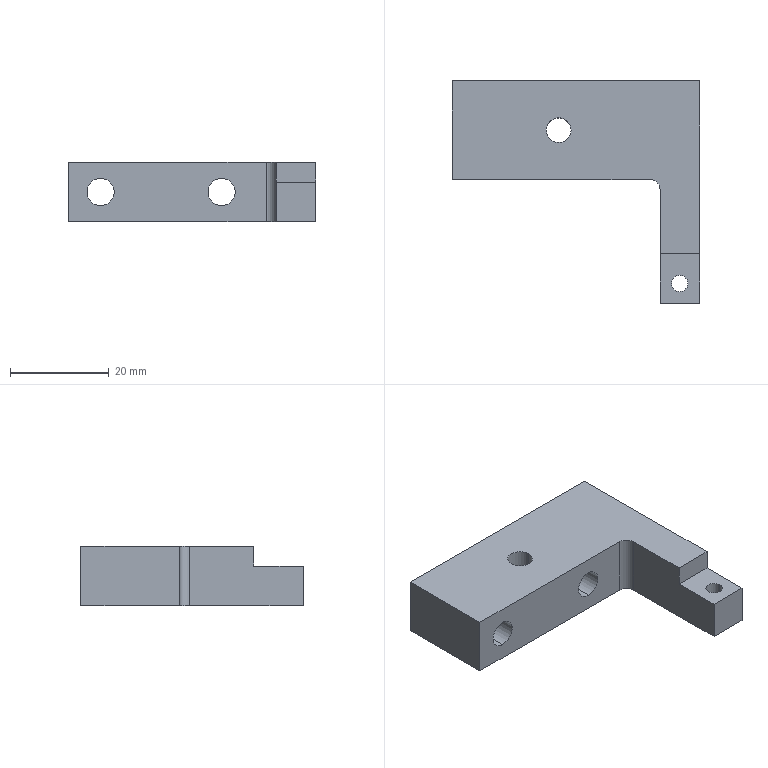Part | STEP file | 11-FG-B05211 | 1 solid | 19 faces | box 50 x 45 x 12 mm | volume 12836 mm3 | plane 10 | cylinder 9 | commonest cylinder face diameters 5.5 x4 3.3 x2 5 x2 4 x1
STEP:
#1=CARTESIAN_POINT('',(24.,10.,0.));
#2=VERTEX_POINT('',#1);
#3=CARTESIAN_POINT('',(19.,10.,0.));
#4=VERTEX_POINT('',#3);
#5=CARTESIAN_POINT('',(21.5,10.,0.));
#6=DIRECTION('',(0.,0.,-1.));
#7=DIRECTION('',(-1.,0.,0.));
#8=AXIS2_PLACEMENT_3D('',#5,#6,#7);
#9=CIRCLE('',#8,2.5);
#10=EDGE_CURVE('',#2,#4,#9,.T.);
#11=ORIENTED_EDGE('',*,*,#10,.T.);
#12=CARTESIAN_POINT('',(19.,10.,12.));
#13=VERTEX_POINT('',#12);
#14=CARTESIAN_POINT('',(19.,10.,12.));
#15=DIRECTION('',(0.,0.,1.));
#16=VECTOR('',#15,1000.);
#17=LINE('',#14,#16);
#18=EDGE_CURVE('',#4,#13,#17,.T.);
#19=ORIENTED_EDGE('',*,*,#18,.T.);
#20=CARTESIAN_POINT('',(24.,10.,12.));
#21=VERTEX_POINT('',#20);
#22=CARTESIAN_POINT('',(21.5,10.,12.));
#23=DIRECTION('',(0.,0.,1.));
#24=DIRECTION('',(1.,0.,0.));
#25=AXIS2_PLACEMENT_3D('',#22,#23,#24);
#26=CIRCLE('',#25,2.5);
#27=EDGE_CURVE('',#13,#21,#26,.T.);
#28=ORIENTED_EDGE('',*,*,#27,.T.);
#29=CARTESIAN_POINT('',(24.,10.,12.));
#30=DIRECTION('',(0.,0.,1.));
#31=VECTOR('',#30,1000.);
#32=LINE('',#29,#31);
#33=EDGE_CURVE('',#2,#21,#32,.T.);
#34=ORIENTED_EDGE('',*,*,#33,.F.);
#35=EDGE_LOOP('',(#11,#19,#28,#34));
#36=FACE_OUTER_BOUND('',#35,.T.);
#37=CARTESIAN_POINT('',(21.5,10.,12.));
#38=DIRECTION('',(0.,0.,1.));
#39=DIRECTION('',(1.,0.,0.));
#40=AXIS2_PLACEMENT_3D('',#37,#38,#39);
#41=CYLINDRICAL_SURFACE('',#40,2.5);
#42=ADVANCED_FACE('',(#36),#41,.F.);
#43=CARTESIAN_POINT('',(31.,20.,8.75));
#44=VERTEX_POINT('',#43);
#45=CARTESIAN_POINT('',(31.,20.,3.25));
#46=VERTEX_POINT('',#45);
#47=CARTESIAN_POINT('',(31.,20.,6.));
#48=DIRECTION('',(0.,-1.,0.));
#49=DIRECTION('',(0.,0.,-1.));
#50=AXIS2_PLACEMENT_3D('',#47,#48,#49);
#51=CIRCLE('',#50,2.75);
#52=EDGE_CURVE('',#44,#46,#51,.T.);
#53=ORIENTED_EDGE('',*,*,#52,.F.);
#54=CARTESIAN_POINT('',(31.,0.,8.75));
#55=VERTEX_POINT('',#54);
#56=CARTESIAN_POINT('',(31.,28.,8.75));
#57=DIRECTION('',(0.,-1.,0.));
#58=VECTOR('',#57,1000.);
#59=LINE('',#56,#58);
#60=EDGE_CURVE('',#44,#55,#59,.T.);
#61=ORIENTED_EDGE('',*,*,#60,.T.);
#62=CARTESIAN_POINT('',(31.,0.,3.25));
#63=VERTEX_POINT('',#62);
#64=CARTESIAN_POINT('',(31.,0.,6.));
#65=DIRECTION('',(0.,-1.,0.));
#66=DIRECTION('',(0.,0.,-1.));
#67=AXIS2_PLACEMENT_3D('',#64,#65,#66);
#68=CIRCLE('',#67,2.75);
#69=EDGE_CURVE('',#55,#63,#68,.T.);
#70=ORIENTED_EDGE('',*,*,#69,.T.);
#71=CARTESIAN_POINT('',(31.,28.,3.25));
#72=DIRECTION('',(0.,-1.,0.));
#73=VECTOR('',#72,1000.);
#74=LINE('',#71,#73);
#75=EDGE_CURVE('',#46,#63,#74,.T.);
#76=ORIENTED_EDGE('',*,*,#75,.F.);
#77=EDGE_LOOP('',(#53,#61,#70,#76));
#78=FACE_OUTER_BOUND('',#77,.T.);
#79=CARTESIAN_POINT('',(31.,28.,6.));
#80=DIRECTION('',(0.,-1.,0.));
#81=DIRECTION('',(0.,0.,-1.));
#82=AXIS2_PLACEMENT_3D('',#79,#80,#81);
#83=CYLINDRICAL_SURFACE('',#82,2.75);
#84=ADVANCED_FACE('',(#78),#83,.F.);
#85=CARTESIAN_POINT('',(6.5,20.,8.75));
#86=VERTEX_POINT('',#85);
#87=CARTESIAN_POINT('',(6.5,20.,3.25));
#88=VERTEX_POINT('',#87);
#89=CARTESIAN_POINT('',(6.5,20.,6.));
#90=DIRECTION('',(0.,-1.,0.));
#91=DIRECTION('',(0.,0.,-1.));
#92=AXIS2_PLACEMENT_3D('',#89,#90,#91);
#93=CIRCLE('',#92,2.75);
#94=EDGE_CURVE('',#86,#88,#93,.T.);
#95=ORIENTED_EDGE('',*,*,#94,.F.);
#96=CARTESIAN_POINT('',(6.5,0.,8.75));
#97=VERTEX_POINT('',#96);
#98=CARTESIAN_POINT('',(6.5,28.,8.75));
#99=DIRECTION('',(0.,-1.,0.));
#100=VECTOR('',#99,1000.);
#101=LINE('',#98,#100);
#102=EDGE_CURVE('',#86,#97,#101,.T.);
#103=ORIENTED_EDGE('',*,*,#102,.T.);
#104=CARTESIAN_POINT('',(6.5,0.,3.25));
#105=VERTEX_POINT('',#104);
#106=CARTESIAN_POINT('',(6.5,0.,6.));
#107=DIRECTION('',(0.,-1.,0.));
#108=DIRECTION('',(0.,0.,-1.));
#109=AXIS2_PLACEMENT_3D('',#106,#107,#108);
#110=CIRCLE('',#109,2.75);
#111=EDGE_CURVE('',#97,#105,#110,.T.);
#112=ORIENTED_EDGE('',*,*,#111,.T.);
#113=CARTESIAN_POINT('',(6.5,28.,3.25));
#114=DIRECTION('',(0.,-1.,0.));
#115=VECTOR('',#114,1000.);
#116=LINE('',#113,#115);
#117=EDGE_CURVE('',#88,#105,#116,.T.);
#118=ORIENTED_EDGE('',*,*,#117,.F.);
#119=EDGE_LOOP('',(#95,#103,#112,#118));
#120=FACE_OUTER_BOUND('',#119,.T.);
#121=CARTESIAN_POINT('',(6.5,28.,6.));
#122=DIRECTION('',(0.,-1.,0.));
#123=DIRECTION('',(0.,0.,-1.));
#124=AXIS2_PLACEMENT_3D('',#121,#122,#123);
#125=CYLINDRICAL_SURFACE('',#124,2.75);
#126=ADVANCED_FACE('',(#120),#125,.F.);
#127=CARTESIAN_POINT('',(47.65,-21.,0.));
#128=VERTEX_POINT('',#127);
#129=CARTESIAN_POINT('',(44.35,-21.,0.));
#130=VERTEX_POINT('',#129);
#131=CARTESIAN_POINT('',(46.,-21.,0.));
#132=DIRECTION('',(0.,0.,-1.));
#133=DIRECTION('',(-1.,0.,0.));
#134=AXIS2_PLACEMENT_3D('',#131,#132,#133);
#135=CIRCLE('',#134,1.65);
#136=EDGE_CURVE('',#128,#130,#135,.T.);
#137=ORIENTED_EDGE('',*,*,#136,.T.);
#138=CARTESIAN_POINT('',(44.35,-21.,8.));
#139=VERTEX_POINT('',#138);
#140=CARTESIAN_POINT('',(44.35,-21.,8.));
#141=DIRECTION('',(0.,0.,1.));
#142=VECTOR('',#141,1000.);
#143=LINE('',#140,#142);
#144=EDGE_CURVE('',#130,#139,#143,.T.);
#145=ORIENTED_EDGE('',*,*,#144,.T.);
#146=CARTESIAN_POINT('',(47.65,-21.,8.));
#147=VERTEX_POINT('',#146);
#148=CARTESIAN_POINT('',(46.,-21.,8.));
#149=DIRECTION('',(0.,0.,1.));
#150=DIRECTION('',(1.,0.,0.));
#151=AXIS2_PLACEMENT_3D('',#148,#149,#150);
#152=CIRCLE('',#151,1.65);
#153=EDGE_CURVE('',#139,#147,#152,.T.);
#154=ORIENTED_EDGE('',*,*,#153,.T.);
#155=CARTESIAN_POINT('',(47.65,-21.,8.));
#156=DIRECTION('',(0.,0.,1.));
#157=VECTOR('',#156,1000.);
#158=LINE('',#155,#157);
#159=EDGE_CURVE('',#128,#147,#158,.T.);
#160=ORIENTED_EDGE('',*,*,#159,.F.);
#161=EDGE_LOOP('',(#137,#145,#154,#160));
#162=FACE_OUTER_BOUND('',#161,.T.);
#163=CARTESIAN_POINT('',(46.,-21.,8.));
#164=DIRECTION('',(0.,0.,1.));
#165=DIRECTION('',(1.,0.,0.));
#166=AXIS2_PLACEMENT_3D('',#163,#164,#165);
#167=CYLINDRICAL_SURFACE('',#166,1.65);
#168=ADVANCED_FACE('',(#162),#167,.F.);
#169=CARTESIAN_POINT('',(50.,-25.,0.));
#170=VERTEX_POINT('',#169);
#171=CARTESIAN_POINT('',(50.,-25.,8.));
#172=VERTEX_POINT('',#171);
#173=CARTESIAN_POINT('',(50.,-25.,0.));
#174=DIRECTION('',(0.,0.,1.));
#175=VECTOR('',#174,1000.);
#176=LINE('',#173,#175);
#177=EDGE_CURVE('',#170,#172,#176,.T.);
#178=ORIENTED_EDGE('',*,*,#177,.T.);
#179=CARTESIAN_POINT('',(42.,-25.,8.));
#180=VERTEX_POINT('',#179);
#181=CARTESIAN_POINT('',(50.,-25.,8.));
#182=DIRECTION('',(1.,0.,0.));
#183=VECTOR('',#182,1000.);
#184=LINE('',#181,#183);
#185=EDGE_CURVE('',#180,#172,#184,.T.);
#186=ORIENTED_EDGE('',*,*,#185,.F.);
#187=CARTESIAN_POINT('',(42.,-25.,0.));
#188=VERTEX_POINT('',#187);
#189=CARTESIAN_POINT('',(42.,-25.,0.));
#190=DIRECTION('',(0.,0.,1.));
#191=VECTOR('',#190,1000.);
#192=LINE('',#189,#191);
#193=EDGE_CURVE('',#188,#180,#192,.T.);
#194=ORIENTED_EDGE('',*,*,#193,.F.);
#195=CARTESIAN_POINT('',(50.,-25.,0.));
#196=DIRECTION('',(1.,0.,0.));
#197=VECTOR('',#196,1000.);
#198=LINE('',#195,#197);
#199=EDGE_CURVE('',#188,#170,#198,.T.);
#200=ORIENTED_EDGE('',*,*,#199,.T.);
#201=EDGE_LOOP('',(#178,#186,#194,#200));
#202=FACE_OUTER_BOUND('',#201,.T.);
#203=CARTESIAN_POINT('',(50.,-25.,0.));
#204=DIRECTION('',(0.,-1.,0.));
#205=DIRECTION('',(0.,0.,-1.));
#206=AXIS2_PLACEMENT_3D('',#203,#204,#205);
#207=PLANE('',#206);
#208=ADVANCED_FACE('',(#202),#207,.T.);
#209=CARTESIAN_POINT('',(0.,20.,0.));
#210=VERTEX_POINT('',#209);
#211=CARTESIAN_POINT('',(0.,0.,0.));
#212=VERTEX_POINT('',#211);
#213=CARTESIAN_POINT('',(0.,0.,0.));
#214=DIRECTION('',(0.,-1.,0.));
#215=VECTOR('',#214,1000.);
#216=LINE('',#213,#215);
#217=EDGE_CURVE('',#210,#212,#216,.T.);
#218=ORIENTED_EDGE('',*,*,#217,.T.);
#219=CARTESIAN_POINT('',(0.,0.,12.));
#220=VERTEX_POINT('',#219);
#221=CARTESIAN_POINT('',(0.,0.,12.));
#222=DIRECTION('',(0.,0.,-1.));
#223=VECTOR('',#222,1000.);
#224=LINE('',#221,#223);
#225=EDGE_CURVE('',#220,#212,#224,.T.);
#226=ORIENTED_EDGE('',*,*,#225,.F.);
#227=CARTESIAN_POINT('',(0.,20.,12.));
#228=VERTEX_POINT('',#227);
#229=CARTESIAN_POINT('',(0.,0.,12.));
#230=DIRECTION('',(0.,-1.,0.));
#231=VECTOR('',#230,1000.);
#232=LINE('',#229,#231);
#233=EDGE_CURVE('',#228,#220,#232,.T.);
#234=ORIENTED_EDGE('',*,*,#233,.F.);
#235=CARTESIAN_POINT('',(0.,20.,12.));
#236=DIRECTION('',(0.,0.,-1.));
#237=VECTOR('',#236,1000.);
#238=LINE('',#235,#237);
#239=EDGE_CURVE('',#228,#210,#238,.T.);
#240=ORIENTED_EDGE('',*,*,#239,.T.);
#241=EDGE_LOOP('',(#218,#226,#234,#240));
#242=FACE_OUTER_BOUND('',#241,.T.);
#243=CARTESIAN_POINT('',(0.,0.,12.));
#244=DIRECTION('',(1.,0.,0.));
#245=DIRECTION('',(0.,0.,-1.));
#246=AXIS2_PLACEMENT_3D('',#243,#244,#245);
#247=PLANE('',#246);
#248=ADVANCED_FACE('',(#242),#247,.F.);
#249=CARTESIAN_POINT('',(31.,0.,6.));
#250=DIRECTION('',(0.,-1.,0.));
#251=DIRECTION('',(0.,0.,-1.));
#252=AXIS2_PLACEMENT_3D('',#249,#250,#251);
#253=CIRCLE('',#252,2.75);
#254=EDGE_CURVE('',#63,#55,#253,.T.);
#255=ORIENTED_EDGE('',*,*,#254,.F.);
#256=ORIENTED_EDGE('',*,*,#69,.F.);
#257=EDGE_LOOP('',(#255,#256));
#258=FACE_BOUND('',#257,.T.);
#259=CARTESIAN_POINT('',(6.5,0.,6.));
#260=DIRECTION('',(0.,-1.,0.));
#261=DIRECTION('',(0.,0.,-1.));
#262=AXIS2_PLACEMENT_3D('',#259,#260,#261);
#263=CIRCLE('',#262,2.75);
#264=EDGE_CURVE('',#105,#97,#263,.T.);
#265=ORIENTED_EDGE('',*,*,#264,.F.);
#266=ORIENTED_EDGE('',*,*,#111,.F.);
#267=EDGE_LOOP('',(#265,#266));
#268=FACE_BOUND('',#267,.T.);
#269=CARTESIAN_POINT('',(40.,0.,0.));
#270=VERTEX_POINT('',#269);
#271=CARTESIAN_POINT('',(0.,0.,0.));
#272=DIRECTION('',(1.,0.,0.));
#273=VECTOR('',#272,1000.);
#274=LINE('',#271,#273);
#275=EDGE_CURVE('',#212,#270,#274,.T.);
#276=ORIENTED_EDGE('',*,*,#275,.T.);
#277=CARTESIAN_POINT('',(40.,0.,12.));
#278=VERTEX_POINT('',#277);
#279=CARTESIAN_POINT('',(40.,0.,12.));
#280=DIRECTION('',(0.,0.,1.));
#281=VECTOR('',#280,1000.);
#282=LINE('',#279,#281);
#283=EDGE_CURVE('',#270,#278,#282,.T.);
#284=ORIENTED_EDGE('',*,*,#283,.T.);
#285=CARTESIAN_POINT('',(0.,0.,12.));
#286=DIRECTION('',(1.,0.,0.));
#287=VECTOR('',#286,1000.);
#288=LINE('',#285,#287);
#289=EDGE_CURVE('',#220,#278,#288,.T.);
#290=ORIENTED_EDGE('',*,*,#289,.F.);
#291=ORIENTED_EDGE('',*,*,#225,.T.);
#292=EDGE_LOOP('',(#276,#284,#290,#291));
#293=FACE_OUTER_BOUND('',#292,.T.);
#294=CARTESIAN_POINT('',(0.,0.,12.));
#295=DIRECTION('',(0.,1.,0.));
#296=DIRECTION('',(0.,0.,1.));
#297=AXIS2_PLACEMENT_3D('',#294,#295,#296);
#298=PLANE('',#297);
#299=ADVANCED_FACE('',(#258,#268,#293),#298,.F.);
#300=CARTESIAN_POINT('',(50.,-15.,12.));
#301=VERTEX_POINT('',#300);
#302=CARTESIAN_POINT('',(50.,20.,12.));
#303=VERTEX_POINT('',#302);
#304=CARTESIAN_POINT('',(50.,0.,12.));
#305=DIRECTION('',(0.,1.,0.));
#306=VECTOR('',#305,1000.);
#307=LINE('',#304,#306);
#308=EDGE_CURVE('',#301,#303,#307,.T.);
#309=ORIENTED_EDGE('',*,*,#308,.F.);
#310=CARTESIAN_POINT('',(50.,-15.,8.));
#311=VERTEX_POINT('',#310);
#312=CARTESIAN_POINT('',(50.,-15.,8.));
#313=DIRECTION('',(0.,0.,1.));
#314=VECTOR('',#313,1000.);
#315=LINE('',#312,#314);
#316=EDGE_CURVE('',#311,#301,#315,.T.);
#317=ORIENTED_EDGE('',*,*,#316,.F.);
#318=CARTESIAN_POINT('',(50.,-25.,8.));
#319=DIRECTION('',(0.,1.,0.));
#320=VECTOR('',#319,1000.);
#321=LINE('',#318,#320);
#322=EDGE_CURVE('',#172,#311,#321,.T.);
#323=ORIENTED_EDGE('',*,*,#322,.F.);
#324=ORIENTED_EDGE('',*,*,#177,.F.);
#325=CARTESIAN_POINT('',(50.,20.,0.));
#326=VERTEX_POINT('',#325);
#327=CARTESIAN_POINT('',(50.,0.,0.));
#328=DIRECTION('',(0.,1.,0.));
#329=VECTOR('',#328,1000.);
#330=LINE('',#327,#329);
#331=EDGE_CURVE('',#170,#326,#330,.T.);
#332=ORIENTED_EDGE('',*,*,#331,.T.);
#333=CARTESIAN_POINT('',(50.,20.,12.));
#334=DIRECTION('',(0.,0.,-1.));
#335=VECTOR('',#334,1000.);
#336=LINE('',#333,#335);
#337=EDGE_CURVE('',#303,#326,#336,.T.);
#338=ORIENTED_EDGE('',*,*,#337,.F.);
#339=EDGE_LOOP('',(#309,#317,#323,#324,#332,#338));
#340=FACE_OUTER_BOUND('',#339,.T.);
#341=CARTESIAN_POINT('',(50.,0.,12.));
#342=DIRECTION('',(-1.,0.,0.));
#343=DIRECTION('',(0.,-1.,0.));
#344=AXIS2_PLACEMENT_3D('',#341,#342,#343);
#345=PLANE('',#344);
#346=ADVANCED_FACE('',(#340),#345,.F.);
#347=CARTESIAN_POINT('',(31.,20.,6.));
#348=DIRECTION('',(0.,-1.,0.));
#349=DIRECTION('',(0.,0.,-1.));
#350=AXIS2_PLACEMENT_3D('',#347,#348,#349);
#351=CIRCLE('',#350,2.75);
#352=EDGE_CURVE('',#46,#44,#351,.T.);
#353=ORIENTED_EDGE('',*,*,#352,.T.);
#354=ORIENTED_EDGE('',*,*,#52,.T.);
#355=EDGE_LOOP('',(#353,#354));
#356=FACE_BOUND('',#355,.T.);
#357=CARTESIAN_POINT('',(6.5,20.,6.));
#358=DIRECTION('',(0.,-1.,0.));
#359=DIRECTION('',(0.,0.,-1.));
#360=AXIS2_PLACEMENT_3D('',#357,#358,#359);
#361=CIRCLE('',#360,2.75);
#362=EDGE_CURVE('',#88,#86,#361,.T.);
#363=ORIENTED_EDGE('',*,*,#362,.T.);
#364=ORIENTED_EDGE('',*,*,#94,.T.);
#365=EDGE_LOOP('',(#363,#364));
#366=FACE_BOUND('',#365,.T.);
#367=CARTESIAN_POINT('',(0.,20.,0.));
#368=DIRECTION('',(-1.,0.,0.));
#369=VECTOR('',#368,1000.);
#370=LINE('',#367,#369);
#371=EDGE_CURVE('',#326,#210,#370,.T.);
#372=ORIENTED_EDGE('',*,*,#371,.T.);
#373=ORIENTED_EDGE('',*,*,#239,.F.);
#374=CARTESIAN_POINT('',(0.,20.,12.));
#375=DIRECTION('',(-1.,0.,0.));
#376=VECTOR('',#375,1000.);
#377=LINE('',#374,#376);
#378=EDGE_CURVE('',#303,#228,#377,.T.);
#379=ORIENTED_EDGE('',*,*,#378,.F.);
#380=ORIENTED_EDGE('',*,*,#337,.T.);
#381=EDGE_LOOP('',(#372,#373,#379,#380));
#382=FACE_OUTER_BOUND('',#381,.T.);
#383=CARTESIAN_POINT('',(0.,20.,12.));
#384=DIRECTION('',(0.,-1.,0.));
#385=DIRECTION('',(0.,0.,-1.));
#386=AXIS2_PLACEMENT_3D('',#383,#384,#385);
#387=PLANE('',#386);
#388=ADVANCED_FACE('',(#356,#366,#382),#387,.F.);
#389=CARTESIAN_POINT('',(21.5,10.,12.));
#390=DIRECTION('',(0.,0.,1.));
#391=DIRECTION('',(1.,0.,0.));
#392=AXIS2_PLACEMENT_3D('',#389,#390,#391);
#393=CIRCLE('',#392,2.5);
#394=EDGE_CURVE('',#21,#13,#393,.T.);
#395=ORIENTED_EDGE('',*,*,#394,.F.);
#396=ORIENTED_EDGE('',*,*,#27,.F.);
#397=EDGE_LOOP('',(#395,#396));
#398=FACE_BOUND('',#397,.T.);
#399=ORIENTED_EDGE('',*,*,#289,.T.);
#400=CARTESIAN_POINT('',(42.,-2.,12.));
#401=VERTEX_POINT('',#400);
#402=CARTESIAN_POINT('',(40.,-2.,12.));
#403=DIRECTION('',(0.,0.,-1.));
#404=DIRECTION('',(-1.,0.,0.));
#405=AXIS2_PLACEMENT_3D('',#402,#403,#404);
#406=CIRCLE('',#405,2.);
#407=EDGE_CURVE('',#278,#401,#406,.T.);
#408=ORIENTED_EDGE('',*,*,#407,.T.);
#409=CARTESIAN_POINT('',(42.,-15.,12.));
#410=VERTEX_POINT('',#409);
#411=CARTESIAN_POINT('',(42.,0.,12.));
#412=DIRECTION('',(0.,-1.,0.));
#413=VECTOR('',#412,1000.);
#414=LINE('',#411,#413);
#415=EDGE_CURVE('',#401,#410,#414,.T.);
#416=ORIENTED_EDGE('',*,*,#415,.T.);
#417=CARTESIAN_POINT('',(50.,-15.,12.));
#418=DIRECTION('',(-1.,0.,0.));
#419=VECTOR('',#418,1000.);
#420=LINE('',#417,#419);
#421=EDGE_CURVE('',#301,#410,#420,.T.);
#422=ORIENTED_EDGE('',*,*,#421,.F.);
#423=ORIENTED_EDGE('',*,*,#308,.T.);
#424=ORIENTED_EDGE('',*,*,#378,.T.);
#425=ORIENTED_EDGE('',*,*,#233,.T.);
#426=EDGE_LOOP('',(#399,#408,#416,#422,#423,#424,#425));
#427=FACE_OUTER_BOUND('',#426,.T.);
#428=CARTESIAN_POINT('',(0.,20.,12.));
#429=DIRECTION('',(0.,0.,-1.));
#430=DIRECTION('',(-1.,0.,0.));
#431=AXIS2_PLACEMENT_3D('',#428,#429,#430);
#432=PLANE('',#431);
#433=ADVANCED_FACE('',(#398,#427),#432,.F.);
#434=ORIENTED_EDGE('',*,*,#10,.F.);
#435=CARTESIAN_POINT('',(21.5,10.,0.));
#436=DIRECTION('',(0.,0.,-1.));
#437=DIRECTION('',(-1.,0.,0.));
#438=AXIS2_PLACEMENT_3D('',#435,#436,#437);
#439=CIRCLE('',#438,2.5);
#440=EDGE_CURVE('',#4,#2,#439,.T.);
#441=ORIENTED_EDGE('',*,*,#440,.F.);
#442=EDGE_LOOP('',(#434,#441));
#443=FACE_BOUND('',#442,.T.);
#444=ORIENTED_EDGE('',*,*,#136,.F.);
#445=CARTESIAN_POINT('',(46.,-21.,0.));
#446=DIRECTION('',(0.,0.,-1.));
#447=DIRECTION('',(-1.,0.,0.));
#448=AXIS2_PLACEMENT_3D('',#445,#446,#447);
#449=CIRCLE('',#448,1.65);
#450=EDGE_CURVE('',#130,#128,#449,.T.);
#451=ORIENTED_EDGE('',*,*,#450,.F.);
#452=EDGE_LOOP('',(#444,#451));
#453=FACE_BOUND('',#452,.T.);
#454=ORIENTED_EDGE('',*,*,#217,.F.);
#455=ORIENTED_EDGE('',*,*,#371,.F.);
#456=ORIENTED_EDGE('',*,*,#331,.F.);
#457=ORIENTED_EDGE('',*,*,#199,.F.);
#458=CARTESIAN_POINT('',(42.,-2.,0.));
#459=VERTEX_POINT('',#458);
#460=CARTESIAN_POINT('',(42.,0.,0.));
#461=DIRECTION('',(0.,-1.,0.));
#462=VECTOR('',#461,1000.);
#463=LINE('',#460,#462);
#464=EDGE_CURVE('',#459,#188,#463,.T.);
#465=ORIENTED_EDGE('',*,*,#464,.F.);
#466=CARTESIAN_POINT('',(40.,-2.,0.));
#467=DIRECTION('',(0.,0.,1.));
#468=DIRECTION('',(-1.,0.,0.));
#469=AXIS2_PLACEMENT_3D('',#466,#467,#468);
#470=CIRCLE('',#469,2.);
#471=EDGE_CURVE('',#459,#270,#470,.T.);
#472=ORIENTED_EDGE('',*,*,#471,.T.);
#473=ORIENTED_EDGE('',*,*,#275,.F.);
#474=EDGE_LOOP('',(#454,#455,#456,#457,#465,#472,#473));
#475=FACE_OUTER_BOUND('',#474,.T.);
#476=CARTESIAN_POINT('',(0.,20.,0.));
#477=DIRECTION('',(0.,0.,-1.));
#478=DIRECTION('',(-1.,0.,0.));
#479=AXIS2_PLACEMENT_3D('',#476,#477,#478);
#480=PLANE('',#479);
#481=ADVANCED_FACE('',(#443,#453,#475),#480,.T.);
#482=ORIENTED_EDGE('',*,*,#415,.F.);
#483=CARTESIAN_POINT('',(42.,-2.,0.));
#484=DIRECTION('',(0.,0.,-1.));
#485=VECTOR('',#484,1000.);
#486=LINE('',#483,#485);
#487=EDGE_CURVE('',#401,#459,#486,.T.);
#488=ORIENTED_EDGE('',*,*,#487,.T.);
#489=ORIENTED_EDGE('',*,*,#464,.T.);
#490=ORIENTED_EDGE('',*,*,#193,.T.);
#491=CARTESIAN_POINT('',(42.,-15.,8.));
#492=VERTEX_POINT('',#491);
#493=CARTESIAN_POINT('',(42.,-25.,8.));
#494=DIRECTION('',(0.,-1.,0.));
#495=VECTOR('',#494,1000.);
#496=LINE('',#493,#495);
#497=EDGE_CURVE('',#492,#180,#496,.T.);
#498=ORIENTED_EDGE('',*,*,#497,.F.);
#499=CARTESIAN_POINT('',(42.,-15.,8.));
#500=DIRECTION('',(0.,0.,1.));
#501=VECTOR('',#500,1000.);
#502=LINE('',#499,#501);
#503=EDGE_CURVE('',#492,#410,#502,.T.);
#504=ORIENTED_EDGE('',*,*,#503,.T.);
#505=EDGE_LOOP('',(#482,#488,#489,#490,#498,#504));
#506=FACE_OUTER_BOUND('',#505,.T.);
#507=CARTESIAN_POINT('',(42.,0.,0.));
#508=DIRECTION('',(-1.,0.,0.));
#509=DIRECTION('',(0.,-1.,0.));
#510=AXIS2_PLACEMENT_3D('',#507,#508,#509);
#511=PLANE('',#510);
#512=ADVANCED_FACE('',(#506),#511,.T.);
#513=ORIENTED_EDGE('',*,*,#421,.T.);
#514=ORIENTED_EDGE('',*,*,#503,.F.);
#515=CARTESIAN_POINT('',(50.,-15.,8.));
#516=DIRECTION('',(-1.,0.,0.));
#517=VECTOR('',#516,1000.);
#518=LINE('',#515,#517);
#519=EDGE_CURVE('',#311,#492,#518,.T.);
#520=ORIENTED_EDGE('',*,*,#519,.F.);
#521=ORIENTED_EDGE('',*,*,#316,.T.);
#522=EDGE_LOOP('',(#513,#514,#520,#521));
#523=FACE_OUTER_BOUND('',#522,.T.);
#524=CARTESIAN_POINT('',(50.,-15.,8.));
#525=DIRECTION('',(0.,1.,0.));
#526=DIRECTION('',(0.,0.,1.));
#527=AXIS2_PLACEMENT_3D('',#524,#525,#526);
#528=PLANE('',#527);
#529=ADVANCED_FACE('',(#523),#528,.F.);
#530=CARTESIAN_POINT('',(46.,-21.,8.));
#531=DIRECTION('',(0.,0.,1.));
#532=DIRECTION('',(1.,0.,0.));
#533=AXIS2_PLACEMENT_3D('',#530,#531,#532);
#534=CIRCLE('',#533,1.65);
#535=EDGE_CURVE('',#147,#139,#534,.T.);
#536=ORIENTED_EDGE('',*,*,#535,.F.);
#537=ORIENTED_EDGE('',*,*,#153,.F.);
#538=EDGE_LOOP('',(#536,#537));
#539=FACE_BOUND('',#538,.T.);
#540=ORIENTED_EDGE('',*,*,#322,.T.);
#541=ORIENTED_EDGE('',*,*,#519,.T.);
#542=ORIENTED_EDGE('',*,*,#497,.T.);
#543=ORIENTED_EDGE('',*,*,#185,.T.);
#544=EDGE_LOOP('',(#540,#541,#542,#543));
#545=FACE_OUTER_BOUND('',#544,.T.);
#546=CARTESIAN_POINT('',(50.,-15.,8.));
#547=DIRECTION('',(0.,0.,1.));
#548=DIRECTION('',(1.,0.,0.));
#549=AXIS2_PLACEMENT_3D('',#546,#547,#548);
#550=PLANE('',#549);
#551=ADVANCED_FACE('',(#539,#545),#550,.T.);
#552=ORIENTED_EDGE('',*,*,#144,.F.);
#553=ORIENTED_EDGE('',*,*,#450,.T.);
#554=ORIENTED_EDGE('',*,*,#159,.T.);
#555=ORIENTED_EDGE('',*,*,#535,.T.);
#556=EDGE_LOOP('',(#552,#553,#554,#555));
#557=FACE_OUTER_BOUND('',#556,.T.);
#558=CARTESIAN_POINT('',(46.,-21.,8.));
#559=DIRECTION('',(0.,0.,1.));
#560=DIRECTION('',(1.,0.,0.));
#561=AXIS2_PLACEMENT_3D('',#558,#559,#560);
#562=CYLINDRICAL_SURFACE('',#561,1.65);
#563=ADVANCED_FACE('',(#557),#562,.F.);
#564=ORIENTED_EDGE('',*,*,#102,.F.);
#565=ORIENTED_EDGE('',*,*,#362,.F.);
#566=ORIENTED_EDGE('',*,*,#117,.T.);
#567=ORIENTED_EDGE('',*,*,#264,.T.);
#568=EDGE_LOOP('',(#564,#565,#566,#567));
#569=FACE_OUTER_BOUND('',#568,.T.);
#570=CARTESIAN_POINT('',(6.5,28.,6.));
#571=DIRECTION('',(0.,-1.,0.));
#572=DIRECTION('',(0.,0.,-1.));
#573=AXIS2_PLACEMENT_3D('',#570,#571,#572);
#574=CYLINDRICAL_SURFACE('',#573,2.75);
#575=ADVANCED_FACE('',(#569),#574,.F.);
#576=ORIENTED_EDGE('',*,*,#60,.F.);
#577=ORIENTED_EDGE('',*,*,#352,.F.);
#578=ORIENTED_EDGE('',*,*,#75,.T.);
#579=ORIENTED_EDGE('',*,*,#254,.T.);
#580=EDGE_LOOP('',(#576,#577,#578,#579));
#581=FACE_OUTER_BOUND('',#580,.T.);
#582=CARTESIAN_POINT('',(31.,28.,6.));
#583=DIRECTION('',(0.,-1.,0.));
#584=DIRECTION('',(0.,0.,-1.));
#585=AXIS2_PLACEMENT_3D('',#582,#583,#584);
#586=CYLINDRICAL_SURFACE('',#585,2.75);
#587=ADVANCED_FACE('',(#581),#586,.F.);
#588=ORIENTED_EDGE('',*,*,#18,.F.);
#589=ORIENTED_EDGE('',*,*,#440,.T.);
#590=ORIENTED_EDGE('',*,*,#33,.T.);
#591=ORIENTED_EDGE('',*,*,#394,.T.);
#592=EDGE_LOOP('',(#588,#589,#590,#591));
#593=FACE_OUTER_BOUND('',#592,.T.);
#594=CARTESIAN_POINT('',(21.5,10.,12.));
#595=DIRECTION('',(0.,0.,1.));
#596=DIRECTION('',(1.,0.,0.));
#597=AXIS2_PLACEMENT_3D('',#594,#595,#596);
#598=CYLINDRICAL_SURFACE('',#597,2.5);
#599=ADVANCED_FACE('',(#593),#598,.F.);
#600=ORIENTED_EDGE('',*,*,#471,.F.);
#601=ORIENTED_EDGE('',*,*,#487,.F.);
#602=ORIENTED_EDGE('',*,*,#407,.F.);
#603=ORIENTED_EDGE('',*,*,#283,.F.);
#604=EDGE_LOOP('',(#600,#601,#602,#603));
#605=FACE_OUTER_BOUND('',#604,.T.);
#606=CARTESIAN_POINT('',(40.,-2.,12.));
#607=DIRECTION('',(0.,0.,1.));
#608=DIRECTION('',(1.,0.,0.));
#609=AXIS2_PLACEMENT_3D('',#606,#607,#608);
#610=CYLINDRICAL_SURFACE('',#609,2.);
#611=ADVANCED_FACE('',(#605),#610,.F.);
#612=CLOSED_SHELL('',(#42,#84,#126,#168,#208,#248,#299,#346,#388,#433,#481,#512,#529,#551,#563,#575,#587,#599,#611));
#613=MANIFOLD_SOLID_BREP('',#612);
#614=CARTESIAN_POINT('',(0.,0.,0.));
#615=DIRECTION('',(0.,0.,1.));
#616=DIRECTION('',(1.,0.,0.));
#617=AXIS2_PLACEMENT_3D('',#614,#615,#616);
#618=(LENGTH_UNIT()NAMED_UNIT(*)SI_UNIT(.MILLI.,.METRE.));
#619=UNCERTAINTY_MEASURE_WITH_UNIT(LENGTH_MEASURE(0.00001),#618,'','');
#620=(NAMED_UNIT(*)PLANE_ANGLE_UNIT()SI_UNIT($,.RADIAN.));
#621=(NAMED_UNIT(*)SI_UNIT($,.STERADIAN.)SOLID_ANGLE_UNIT());
#622=(GEOMETRIC_REPRESENTATION_CONTEXT(3)GLOBAL_UNCERTAINTY_ASSIGNED_CONTEXT((#619))GLOBAL_UNIT_ASSIGNED_CONTEXT((#618,#620,#621))REPRESENTATION_CONTEXT('',''));
#623=ADVANCED_BREP_SHAPE_REPRESENTATION('',(#613,#617),#622);